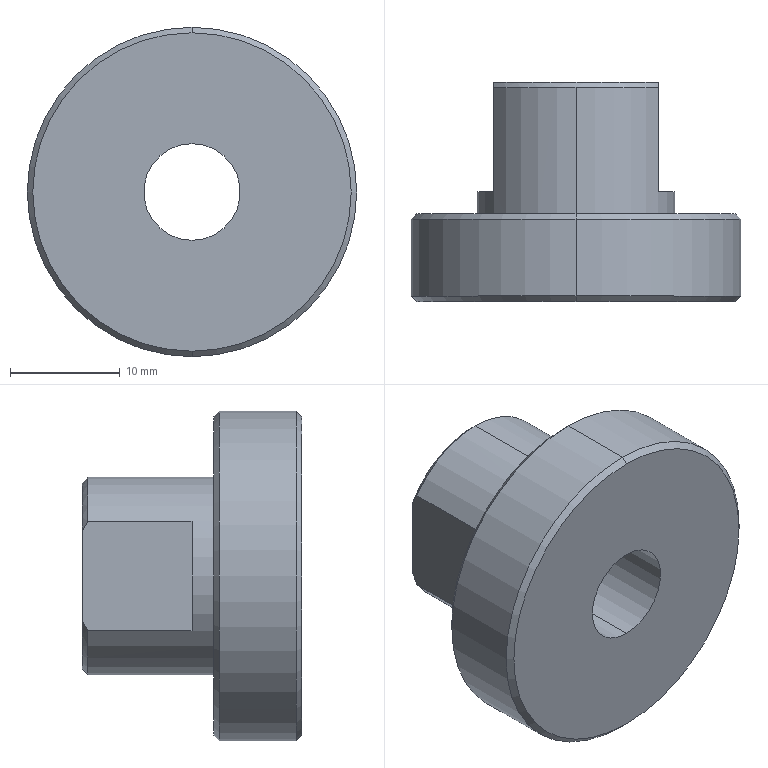Part | STEP file | PN_0022 | 1 solid | 20 faces | box 30 x 20 x 30 mm | volume 7262 mm3 | cone 7 | plane 7 | cylinder 6 | commonest cylinder face diameters 8.8 x2 18 x2 30 x2